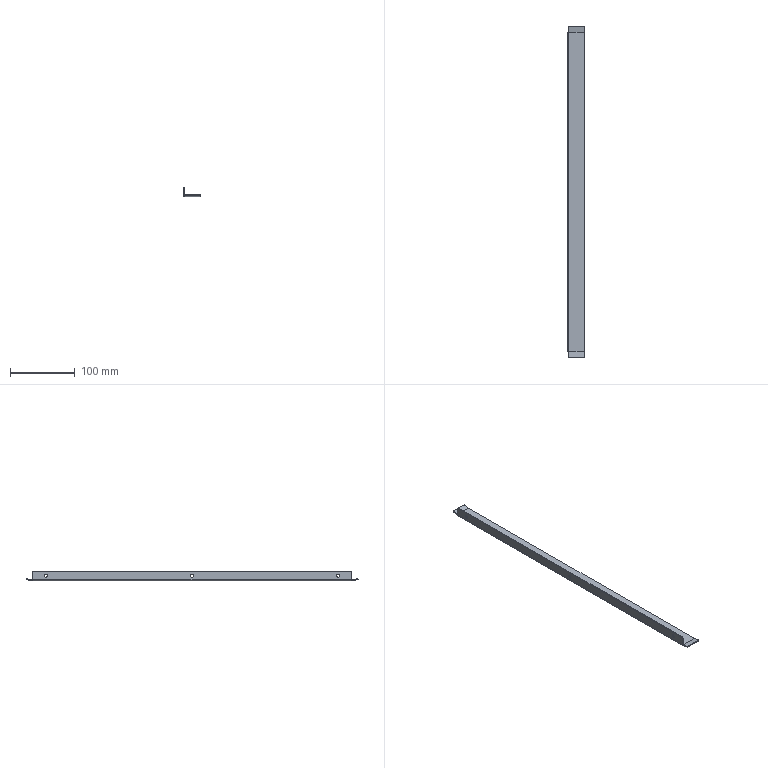Part | STEP file | T10 timing belt support plate | 1 solid | 44 faces | box 25.5 x 510.959 x 15 mm | volume 29071 mm3 | plane 26 | cylinder 18 | commonest cylinder face diameters 4 x6 5 x6 0.1 x3 3.1 x3